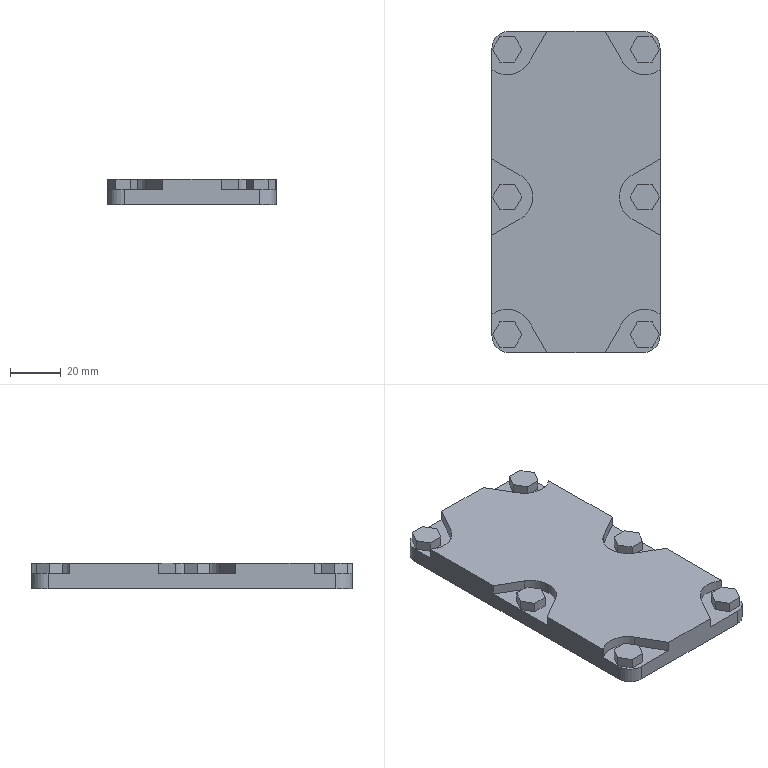Part | SolidWorks | features BaseBody 1 | 1 solid | 73 faces | box 66 x 126 x 10 mm | volume 78056 mm3 | plane 62 | cylinder 11 | commonest cylinder face diameters 20 x7 13 x4